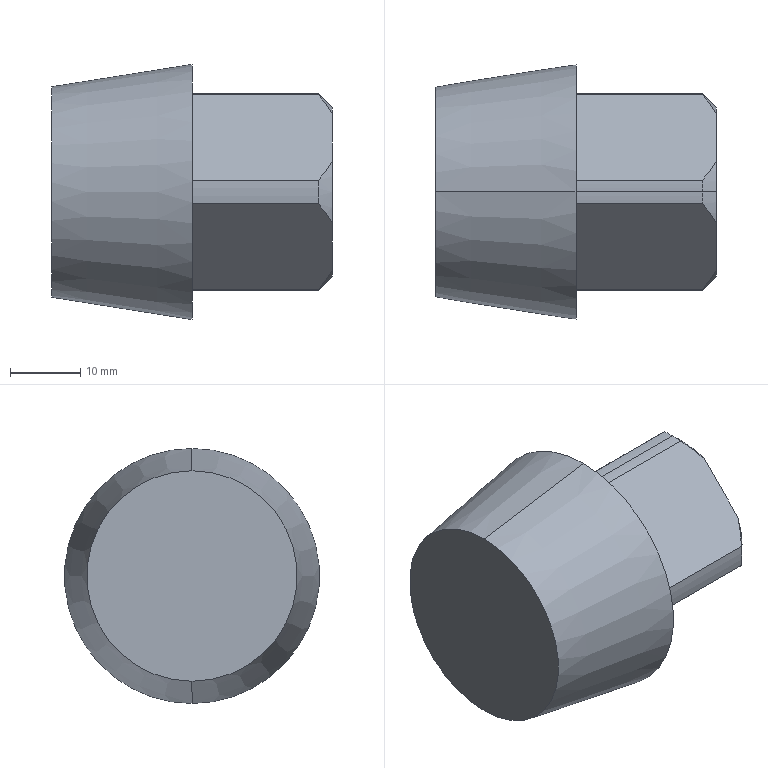Part | SolidWorks | features Chamfer 1, CirPattern 1, ICE 1, Revolution 1 | 1 solid | 19 faces | box 40 x 36.354 x 36.354 mm | volume 26781 mm3 | cone 7 | plane 7 | cylinder 5 | commonest cylinder face diameters 28 x5
STEP:
#1=CARTESIAN_POINT('',(0.,0.,15.));
#2=VERTEX_POINT('',#1);
#3=CARTESIAN_POINT('',(0.,0.,-15.));
#4=VERTEX_POINT('',#3);
#5=CARTESIAN_POINT('',(0.,0.,0.));
#6=DIRECTION('',(-1.,0.,0.));
#7=DIRECTION('',(0.,0.,1.));
#8=AXIS2_PLACEMENT_3D('',#5,#6,#7);
#9=CIRCLE('',#8,15.);
#10=EDGE_CURVE('',#2,#4,#9,.T.);
#11=ORIENTED_EDGE('',*,*,#10,.F.);
#12=CARTESIAN_POINT('',(20.,0.,18.177));
#13=VERTEX_POINT('',#12);
#14=CARTESIAN_POINT('',(20.,0.,18.177));
#15=DIRECTION('',(0.9876,0.,0.1569));
#16=VECTOR('',#15,1000.);
#17=LINE('',#14,#16);
#18=EDGE_CURVE('',#2,#13,#17,.T.);
#19=ORIENTED_EDGE('',*,*,#18,.T.);
#20=CARTESIAN_POINT('',(20.,0.,-18.177));
#21=VERTEX_POINT('',#20);
#22=CARTESIAN_POINT('',(20.,0.,0.));
#23=DIRECTION('',(-1.,0.,0.));
#24=DIRECTION('',(0.,0.,1.));
#25=AXIS2_PLACEMENT_3D('',#22,#23,#24);
#26=CIRCLE('',#25,18.177);
#27=EDGE_CURVE('',#13,#21,#26,.T.);
#28=ORIENTED_EDGE('',*,*,#27,.T.);
#29=CARTESIAN_POINT('',(20.,0.,-18.177));
#30=DIRECTION('',(0.9876,0.,-0.1569));
#31=VECTOR('',#30,1000.);
#32=LINE('',#29,#31);
#33=EDGE_CURVE('',#4,#21,#32,.T.);
#34=ORIENTED_EDGE('',*,*,#33,.F.);
#35=EDGE_LOOP('',(#11,#19,#28,#34));
#36=FACE_OUTER_BOUND('',#35,.T.);
#37=CARTESIAN_POINT('',(20.,0.,0.));
#38=DIRECTION('',(1.,0.,0.));
#39=DIRECTION('',(0.,0.,-1.));
#40=AXIS2_PLACEMENT_3D('',#37,#38,#39);
#41=CONICAL_SURFACE('',#40,18.177,0.1575);
#42=ADVANCED_FACE('',(#36),#41,.T.);
#43=CARTESIAN_POINT('',(40.,0.,12.));
#44=VERTEX_POINT('',#43);
#45=CARTESIAN_POINT('',(40.,-4.387,11.169));
#46=VERTEX_POINT('',#45);
#47=CARTESIAN_POINT('',(40.,0.,0.));
#48=DIRECTION('',(1.,0.,0.));
#49=DIRECTION('',(0.,0.,1.));
#50=AXIS2_PLACEMENT_3D('',#47,#48,#49);
#51=CIRCLE('',#50,12.);
#52=EDGE_CURVE('',#44,#46,#51,.T.);
#53=ORIENTED_EDGE('',*,*,#52,.F.);
#54=CARTESIAN_POINT('',(38.,0.,14.));
#55=VERTEX_POINT('',#54);
#56=CARTESIAN_POINT('',(38.,0.,14.));
#57=DIRECTION('',(-0.7071,0.,0.7071));
#58=VECTOR('',#57,1000.);
#59=LINE('',#56,#58);
#60=EDGE_CURVE('',#44,#55,#59,.T.);
#61=ORIENTED_EDGE('',*,*,#60,.T.);
#62=CARTESIAN_POINT('',(38.,-1.654,13.902));
#63=VERTEX_POINT('',#62);
#64=CARTESIAN_POINT('',(38.,0.,0.));
#65=DIRECTION('',(-1.,0.,0.));
#66=DIRECTION('',(0.,0.,1.));
#67=AXIS2_PLACEMENT_3D('',#64,#65,#66);
#68=CIRCLE('',#67,14.);
#69=EDGE_CURVE('',#63,#55,#68,.T.);
#70=ORIENTED_EDGE('',*,*,#69,.F.);
#71=CARTESIAN_POINT('',(38.,-1.654,13.902));
#72=CARTESIAN_POINT('',(38.384,-2.093,13.463));
#73=CARTESIAN_POINT('',(38.748,-2.538,13.018));
#74=CARTESIAN_POINT('',(39.421,-3.447,12.109));
#75=CARTESIAN_POINT('',(39.731,-3.91,11.646));
#76=CARTESIAN_POINT('',(40.,-4.387,11.169));
#77=B_SPLINE_CURVE_WITH_KNOTS('',3,(#71,#72,#73,#74,#75,#76),.UNSPECIFIED.,.F.,.F.,(4,2,4),(0.000001156,0.002175,0.004349),.UNSPECIFIED.);
#78=EDGE_CURVE('',#63,#46,#77,.T.);
#79=ORIENTED_EDGE('',*,*,#78,.T.);
#80=EDGE_LOOP('',(#53,#61,#70,#79));
#81=FACE_OUTER_BOUND('',#80,.T.);
#82=CARTESIAN_POINT('',(38.,0.,0.));
#83=DIRECTION('',(-1.,0.,0.));
#84=DIRECTION('',(0.,0.,1.));
#85=AXIS2_PLACEMENT_3D('',#82,#83,#84);
#86=CONICAL_SURFACE('',#85,14.,0.7854);
#87=ADVANCED_FACE('',(#81),#86,.T.);
#88=ORIENTED_EDGE('',*,*,#69,.T.);
#89=CARTESIAN_POINT('',(20.,0.,14.));
#90=VERTEX_POINT('',#89);
#91=CARTESIAN_POINT('',(20.,0.,14.));
#92=DIRECTION('',(-1.,0.,0.));
#93=VECTOR('',#92,1000.);
#94=LINE('',#91,#93);
#95=EDGE_CURVE('',#55,#90,#94,.T.);
#96=ORIENTED_EDGE('',*,*,#95,.T.);
#97=CARTESIAN_POINT('',(20.,-1.654,13.902));
#98=VERTEX_POINT('',#97);
#99=CARTESIAN_POINT('',(20.,0.,0.));
#100=DIRECTION('',(-1.,0.,0.));
#101=DIRECTION('',(0.,0.,1.));
#102=AXIS2_PLACEMENT_3D('',#99,#100,#101);
#103=CIRCLE('',#102,14.);
#104=EDGE_CURVE('',#98,#90,#103,.T.);
#105=ORIENTED_EDGE('',*,*,#104,.F.);
#106=CARTESIAN_POINT('',(20.,-1.654,13.902));
#107=DIRECTION('',(1.,0.,0.));
#108=VECTOR('',#107,1000.);
#109=LINE('',#106,#108);
#110=EDGE_CURVE('',#98,#63,#109,.T.);
#111=ORIENTED_EDGE('',*,*,#110,.T.);
#112=EDGE_LOOP('',(#88,#96,#105,#111));
#113=FACE_OUTER_BOUND('',#112,.T.);
#114=CARTESIAN_POINT('',(20.,0.,0.));
#115=DIRECTION('',(-1.,0.,0.));
#116=DIRECTION('',(0.,0.,1.));
#117=AXIS2_PLACEMENT_3D('',#114,#115,#116);
#118=CYLINDRICAL_SURFACE('',#117,14.);
#119=ADVANCED_FACE('',(#113),#118,.T.);
#120=CARTESIAN_POINT('',(20.,-13.902,-1.654));
#121=VERTEX_POINT('',#120);
#122=CARTESIAN_POINT('',(38.,-13.902,-1.654));
#123=VERTEX_POINT('',#122);
#124=CARTESIAN_POINT('',(20.,-13.902,-1.654));
#125=DIRECTION('',(1.,0.,0.));
#126=VECTOR('',#125,1000.);
#127=LINE('',#124,#126);
#128=EDGE_CURVE('',#121,#123,#127,.T.);
#129=ORIENTED_EDGE('',*,*,#128,.T.);
#130=CARTESIAN_POINT('',(38.,-13.902,1.654));
#131=VERTEX_POINT('',#130);
#132=CARTESIAN_POINT('',(38.,0.,0.));
#133=DIRECTION('',(-1.,0.,0.));
#134=DIRECTION('',(0.,0.,1.));
#135=AXIS2_PLACEMENT_3D('',#132,#133,#134);
#136=CIRCLE('',#135,14.);
#137=EDGE_CURVE('',#123,#131,#136,.T.);
#138=ORIENTED_EDGE('',*,*,#137,.T.);
#139=CARTESIAN_POINT('',(20.,-13.902,1.654));
#140=VERTEX_POINT('',#139);
#141=CARTESIAN_POINT('',(20.,-13.902,1.654));
#142=DIRECTION('',(1.,0.,0.));
#143=VECTOR('',#142,1000.);
#144=LINE('',#141,#143);
#145=EDGE_CURVE('',#140,#131,#144,.T.);
#146=ORIENTED_EDGE('',*,*,#145,.F.);
#147=CARTESIAN_POINT('',(20.,0.,0.));
#148=DIRECTION('',(-1.,0.,0.));
#149=DIRECTION('',(0.,0.,1.));
#150=AXIS2_PLACEMENT_3D('',#147,#148,#149);
#151=CIRCLE('',#150,14.);
#152=EDGE_CURVE('',#121,#140,#151,.T.);
#153=ORIENTED_EDGE('',*,*,#152,.F.);
#154=EDGE_LOOP('',(#129,#138,#146,#153));
#155=FACE_OUTER_BOUND('',#154,.T.);
#156=CARTESIAN_POINT('',(20.,0.,0.));
#157=DIRECTION('',(-1.,0.,0.));
#158=DIRECTION('',(0.,0.,1.));
#159=AXIS2_PLACEMENT_3D('',#156,#157,#158);
#160=CYLINDRICAL_SURFACE('',#159,14.);
#161=ADVANCED_FACE('',(#155),#160,.T.);
#162=CARTESIAN_POINT('',(20.,-1.654,-13.902));
#163=VERTEX_POINT('',#162);
#164=CARTESIAN_POINT('',(38.,-1.654,-13.902));
#165=VERTEX_POINT('',#164);
#166=CARTESIAN_POINT('',(20.,-1.654,-13.902));
#167=DIRECTION('',(1.,0.,0.));
#168=VECTOR('',#167,1000.);
#169=LINE('',#166,#168);
#170=EDGE_CURVE('',#163,#165,#169,.T.);
#171=ORIENTED_EDGE('',*,*,#170,.F.);
#172=CARTESIAN_POINT('',(20.,1.654,-13.902));
#173=VERTEX_POINT('',#172);
#174=CARTESIAN_POINT('',(20.,0.,0.));
#175=DIRECTION('',(-1.,0.,0.));
#176=DIRECTION('',(0.,0.,1.));
#177=AXIS2_PLACEMENT_3D('',#174,#175,#176);
#178=CIRCLE('',#177,14.);
#179=EDGE_CURVE('',#173,#163,#178,.T.);
#180=ORIENTED_EDGE('',*,*,#179,.F.);
#181=CARTESIAN_POINT('',(38.,1.654,-13.902));
#182=VERTEX_POINT('',#181);
#183=CARTESIAN_POINT('',(20.,1.654,-13.902));
#184=DIRECTION('',(1.,0.,0.));
#185=VECTOR('',#184,1000.);
#186=LINE('',#183,#185);
#187=EDGE_CURVE('',#173,#182,#186,.T.);
#188=ORIENTED_EDGE('',*,*,#187,.T.);
#189=CARTESIAN_POINT('',(38.,0.,0.));
#190=DIRECTION('',(-1.,0.,0.));
#191=DIRECTION('',(0.,0.,1.));
#192=AXIS2_PLACEMENT_3D('',#189,#190,#191);
#193=CIRCLE('',#192,14.);
#194=EDGE_CURVE('',#182,#165,#193,.T.);
#195=ORIENTED_EDGE('',*,*,#194,.T.);
#196=EDGE_LOOP('',(#171,#180,#188,#195));
#197=FACE_OUTER_BOUND('',#196,.T.);
#198=CARTESIAN_POINT('',(20.,0.,0.));
#199=DIRECTION('',(-1.,0.,0.));
#200=DIRECTION('',(0.,0.,1.));
#201=AXIS2_PLACEMENT_3D('',#198,#199,#200);
#202=CYLINDRICAL_SURFACE('',#201,14.);
#203=ADVANCED_FACE('',(#197),#202,.T.);
#204=ORIENTED_EDGE('',*,*,#95,.F.);
#205=CARTESIAN_POINT('',(38.,1.654,13.902));
#206=VERTEX_POINT('',#205);
#207=CARTESIAN_POINT('',(38.,0.,0.));
#208=DIRECTION('',(-1.,0.,0.));
#209=DIRECTION('',(0.,0.,1.));
#210=AXIS2_PLACEMENT_3D('',#207,#208,#209);
#211=CIRCLE('',#210,14.);
#212=EDGE_CURVE('',#55,#206,#211,.T.);
#213=ORIENTED_EDGE('',*,*,#212,.T.);
#214=CARTESIAN_POINT('',(20.,1.654,13.902));
#215=VERTEX_POINT('',#214);
#216=CARTESIAN_POINT('',(20.,1.654,13.902));
#217=DIRECTION('',(1.,0.,0.));
#218=VECTOR('',#217,1000.);
#219=LINE('',#216,#218);
#220=EDGE_CURVE('',#215,#206,#219,.T.);
#221=ORIENTED_EDGE('',*,*,#220,.F.);
#222=CARTESIAN_POINT('',(20.,0.,0.));
#223=DIRECTION('',(-1.,0.,0.));
#224=DIRECTION('',(0.,0.,1.));
#225=AXIS2_PLACEMENT_3D('',#222,#223,#224);
#226=CIRCLE('',#225,14.);
#227=EDGE_CURVE('',#90,#215,#226,.T.);
#228=ORIENTED_EDGE('',*,*,#227,.F.);
#229=EDGE_LOOP('',(#204,#213,#221,#228));
#230=FACE_OUTER_BOUND('',#229,.T.);
#231=CARTESIAN_POINT('',(20.,0.,0.));
#232=DIRECTION('',(-1.,0.,0.));
#233=DIRECTION('',(0.,0.,1.));
#234=AXIS2_PLACEMENT_3D('',#231,#232,#233);
#235=CYLINDRICAL_SURFACE('',#234,14.);
#236=ADVANCED_FACE('',(#230),#235,.T.);
#237=CARTESIAN_POINT('',(20.,13.902,1.654));
#238=VERTEX_POINT('',#237);
#239=CARTESIAN_POINT('',(38.,13.902,1.654));
#240=VERTEX_POINT('',#239);
#241=CARTESIAN_POINT('',(20.,13.902,1.654));
#242=DIRECTION('',(1.,0.,0.));
#243=VECTOR('',#242,1000.);
#244=LINE('',#241,#243);
#245=EDGE_CURVE('',#238,#240,#244,.T.);
#246=ORIENTED_EDGE('',*,*,#245,.T.);
#247=CARTESIAN_POINT('',(38.,13.902,-1.654));
#248=VERTEX_POINT('',#247);
#249=CARTESIAN_POINT('',(38.,0.,0.));
#250=DIRECTION('',(-1.,0.,0.));
#251=DIRECTION('',(0.,0.,1.));
#252=AXIS2_PLACEMENT_3D('',#249,#250,#251);
#253=CIRCLE('',#252,14.);
#254=EDGE_CURVE('',#240,#248,#253,.T.);
#255=ORIENTED_EDGE('',*,*,#254,.T.);
#256=CARTESIAN_POINT('',(20.,13.902,-1.654));
#257=VERTEX_POINT('',#256);
#258=CARTESIAN_POINT('',(20.,13.902,-1.654));
#259=DIRECTION('',(1.,0.,0.));
#260=VECTOR('',#259,1000.);
#261=LINE('',#258,#260);
#262=EDGE_CURVE('',#257,#248,#261,.T.);
#263=ORIENTED_EDGE('',*,*,#262,.F.);
#264=CARTESIAN_POINT('',(20.,0.,0.));
#265=DIRECTION('',(-1.,0.,0.));
#266=DIRECTION('',(0.,0.,1.));
#267=AXIS2_PLACEMENT_3D('',#264,#265,#266);
#268=CIRCLE('',#267,14.);
#269=EDGE_CURVE('',#238,#257,#268,.T.);
#270=ORIENTED_EDGE('',*,*,#269,.F.);
#271=EDGE_LOOP('',(#246,#255,#263,#270));
#272=FACE_OUTER_BOUND('',#271,.T.);
#273=CARTESIAN_POINT('',(20.,0.,0.));
#274=DIRECTION('',(-1.,0.,0.));
#275=DIRECTION('',(0.,0.,1.));
#276=AXIS2_PLACEMENT_3D('',#273,#274,#275);
#277=CYLINDRICAL_SURFACE('',#276,14.);
#278=ADVANCED_FACE('',(#272),#277,.T.);
#279=CARTESIAN_POINT('',(40.,-11.169,-4.387));
#280=VERTEX_POINT('',#279);
#281=CARTESIAN_POINT('',(40.,-4.387,-11.169));
#282=VERTEX_POINT('',#281);
#283=CARTESIAN_POINT('',(40.,-7.778,-7.778));
#284=DIRECTION('',(0.,0.7071,-0.7071));
#285=VECTOR('',#284,1000.);
#286=LINE('',#283,#285);
#287=EDGE_CURVE('',#280,#282,#286,.T.);
#288=ORIENTED_EDGE('',*,*,#287,.T.);
#289=CARTESIAN_POINT('',(40.,4.387,-11.169));
#290=VERTEX_POINT('',#289);
#291=CARTESIAN_POINT('',(40.,0.,0.));
#292=DIRECTION('',(1.,0.,0.));
#293=DIRECTION('',(0.,0.,1.));
#294=AXIS2_PLACEMENT_3D('',#291,#292,#293);
#295=CIRCLE('',#294,12.);
#296=EDGE_CURVE('',#282,#290,#295,.T.);
#297=ORIENTED_EDGE('',*,*,#296,.T.);
#298=CARTESIAN_POINT('',(40.,11.169,-4.387));
#299=VERTEX_POINT('',#298);
#300=CARTESIAN_POINT('',(40.,7.778,-7.778));
#301=DIRECTION('',(0.,0.7071,0.7071));
#302=VECTOR('',#301,1000.);
#303=LINE('',#300,#302);
#304=EDGE_CURVE('',#290,#299,#303,.T.);
#305=ORIENTED_EDGE('',*,*,#304,.T.);
#306=CARTESIAN_POINT('',(40.,11.169,4.387));
#307=VERTEX_POINT('',#306);
#308=CARTESIAN_POINT('',(40.,0.,0.));
#309=DIRECTION('',(1.,0.,0.));
#310=DIRECTION('',(0.,0.,1.));
#311=AXIS2_PLACEMENT_3D('',#308,#309,#310);
#312=CIRCLE('',#311,12.);
#313=EDGE_CURVE('',#299,#307,#312,.T.);
#314=ORIENTED_EDGE('',*,*,#313,.T.);
#315=CARTESIAN_POINT('',(40.,4.387,11.169));
#316=VERTEX_POINT('',#315);
#317=CARTESIAN_POINT('',(40.,7.778,7.778));
#318=DIRECTION('',(0.,-0.7071,0.7071));
#319=VECTOR('',#318,1000.);
#320=LINE('',#317,#319);
#321=EDGE_CURVE('',#307,#316,#320,.T.);
#322=ORIENTED_EDGE('',*,*,#321,.T.);
#323=CARTESIAN_POINT('',(40.,0.,0.));
#324=DIRECTION('',(1.,0.,0.));
#325=DIRECTION('',(0.,0.,1.));
#326=AXIS2_PLACEMENT_3D('',#323,#324,#325);
#327=CIRCLE('',#326,12.);
#328=EDGE_CURVE('',#316,#44,#327,.T.);
#329=ORIENTED_EDGE('',*,*,#328,.T.);
#330=ORIENTED_EDGE('',*,*,#52,.T.);
#331=CARTESIAN_POINT('',(40.,-11.169,4.387));
#332=VERTEX_POINT('',#331);
#333=CARTESIAN_POINT('',(40.,-7.778,7.778));
#334=DIRECTION('',(0.,-0.7071,-0.7071));
#335=VECTOR('',#334,1000.);
#336=LINE('',#333,#335);
#337=EDGE_CURVE('',#46,#332,#336,.T.);
#338=ORIENTED_EDGE('',*,*,#337,.T.);
#339=CARTESIAN_POINT('',(40.,0.,0.));
#340=DIRECTION('',(1.,0.,0.));
#341=DIRECTION('',(0.,0.,1.));
#342=AXIS2_PLACEMENT_3D('',#339,#340,#341);
#343=CIRCLE('',#342,12.);
#344=EDGE_CURVE('',#332,#280,#343,.T.);
#345=ORIENTED_EDGE('',*,*,#344,.T.);
#346=EDGE_LOOP('',(#288,#297,#305,#314,#322,#329,#330,#338,#345));
#347=FACE_OUTER_BOUND('',#346,.T.);
#348=CARTESIAN_POINT('',(40.,0.,0.));
#349=DIRECTION('',(-1.,0.,0.));
#350=DIRECTION('',(0.,0.,1.));
#351=AXIS2_PLACEMENT_3D('',#348,#349,#350);
#352=PLANE('',#351);
#353=ADVANCED_FACE('',(#347),#352,.F.);
#354=ORIENTED_EDGE('',*,*,#137,.F.);
#355=CARTESIAN_POINT('',(38.,-13.902,-1.654));
#356=CARTESIAN_POINT('',(38.384,-13.463,-2.093));
#357=CARTESIAN_POINT('',(38.748,-13.018,-2.538));
#358=CARTESIAN_POINT('',(39.421,-12.109,-3.447));
#359=CARTESIAN_POINT('',(39.731,-11.646,-3.91));
#360=CARTESIAN_POINT('',(40.,-11.169,-4.387));
#361=B_SPLINE_CURVE_WITH_KNOTS('',3,(#355,#356,#357,#358,#359,#360),.UNSPECIFIED.,.F.,.F.,(4,2,4),(0.000001156,0.002175,0.004349),.UNSPECIFIED.);
#362=EDGE_CURVE('',#123,#280,#361,.T.);
#363=ORIENTED_EDGE('',*,*,#362,.T.);
#364=ORIENTED_EDGE('',*,*,#344,.F.);
#365=CARTESIAN_POINT('',(40.,-11.169,4.387));
#366=CARTESIAN_POINT('',(39.73,-11.648,3.909));
#367=CARTESIAN_POINT('',(39.42,-12.111,3.445));
#368=CARTESIAN_POINT('',(38.747,-13.02,2.536));
#369=CARTESIAN_POINT('',(38.383,-13.464,2.092));
#370=CARTESIAN_POINT('',(38.,-13.902,1.654));
#371=B_SPLINE_CURVE_WITH_KNOTS('',3,(#365,#366,#367,#368,#369,#370),.UNSPECIFIED.,.F.,.F.,(4,2,4),(0.01415,0.01632,0.01848),.UNSPECIFIED.);
#372=EDGE_CURVE('',#332,#131,#371,.T.);
#373=ORIENTED_EDGE('',*,*,#372,.T.);
#374=EDGE_LOOP('',(#354,#363,#364,#373));
#375=FACE_OUTER_BOUND('',#374,.T.);
#376=CARTESIAN_POINT('',(38.,0.,0.));
#377=DIRECTION('',(-1.,0.,0.));
#378=DIRECTION('',(0.,0.,1.));
#379=AXIS2_PLACEMENT_3D('',#376,#377,#378);
#380=CONICAL_SURFACE('',#379,14.,0.7854);
#381=ADVANCED_FACE('',(#375),#380,.T.);
#382=ORIENTED_EDGE('',*,*,#296,.F.);
#383=CARTESIAN_POINT('',(40.,-4.387,-11.169));
#384=CARTESIAN_POINT('',(39.73,-3.909,-11.648));
#385=CARTESIAN_POINT('',(39.42,-3.445,-12.111));
#386=CARTESIAN_POINT('',(38.747,-2.536,-13.02));
#387=CARTESIAN_POINT('',(38.383,-2.092,-13.464));
#388=CARTESIAN_POINT('',(38.,-1.654,-13.902));
#389=B_SPLINE_CURVE_WITH_KNOTS('',3,(#383,#384,#385,#386,#387,#388),.UNSPECIFIED.,.F.,.F.,(4,2,4),(0.01415,0.01632,0.01848),.UNSPECIFIED.);
#390=EDGE_CURVE('',#282,#165,#389,.T.);
#391=ORIENTED_EDGE('',*,*,#390,.T.);
#392=ORIENTED_EDGE('',*,*,#194,.F.);
#393=CARTESIAN_POINT('',(38.,1.654,-13.902));
#394=CARTESIAN_POINT('',(38.384,2.093,-13.463));
#395=CARTESIAN_POINT('',(38.748,2.538,-13.018));
#396=CARTESIAN_POINT('',(39.421,3.447,-12.109));
#397=CARTESIAN_POINT('',(39.731,3.91,-11.646));
#398=CARTESIAN_POINT('',(40.,4.387,-11.169));
#399=B_SPLINE_CURVE_WITH_KNOTS('',3,(#393,#394,#395,#396,#397,#398),.UNSPECIFIED.,.F.,.F.,(4,2,4),(0.000001156,0.002175,0.004349),.UNSPECIFIED.);
#400=EDGE_CURVE('',#182,#290,#399,.T.);
#401=ORIENTED_EDGE('',*,*,#400,.T.);
#402=EDGE_LOOP('',(#382,#391,#392,#401));
#403=FACE_OUTER_BOUND('',#402,.T.);
#404=CARTESIAN_POINT('',(38.,0.,0.));
#405=DIRECTION('',(-1.,0.,0.));
#406=DIRECTION('',(0.,0.,1.));
#407=AXIS2_PLACEMENT_3D('',#404,#405,#406);
#408=CONICAL_SURFACE('',#407,14.,0.7854);
#409=ADVANCED_FACE('',(#403),#408,.T.);
#410=ORIENTED_EDGE('',*,*,#60,.F.);
#411=ORIENTED_EDGE('',*,*,#328,.F.);
#412=CARTESIAN_POINT('',(40.,4.387,11.169));
#413=CARTESIAN_POINT('',(39.73,3.909,11.648));
#414=CARTESIAN_POINT('',(39.42,3.445,12.111));
#415=CARTESIAN_POINT('',(38.747,2.536,13.02));
#416=CARTESIAN_POINT('',(38.383,2.092,13.464));
#417=CARTESIAN_POINT('',(38.,1.654,13.902));
#418=B_SPLINE_CURVE_WITH_KNOTS('',3,(#412,#413,#414,#415,#416,#417),.UNSPECIFIED.,.F.,.F.,(4,2,4),(0.01415,0.01632,0.01848),.UNSPECIFIED.);
#419=EDGE_CURVE('',#316,#206,#418,.T.);
#420=ORIENTED_EDGE('',*,*,#419,.T.);
#421=ORIENTED_EDGE('',*,*,#212,.F.);
#422=EDGE_LOOP('',(#410,#411,#420,#421));
#423=FACE_OUTER_BOUND('',#422,.T.);
#424=CARTESIAN_POINT('',(38.,0.,0.));
#425=DIRECTION('',(-1.,0.,0.));
#426=DIRECTION('',(0.,0.,1.));
#427=AXIS2_PLACEMENT_3D('',#424,#425,#426);
#428=CONICAL_SURFACE('',#427,14.,0.7854);
#429=ADVANCED_FACE('',(#423),#428,.T.);
#430=ORIENTED_EDGE('',*,*,#254,.F.);
#431=CARTESIAN_POINT('',(38.,13.902,1.654));
#432=CARTESIAN_POINT('',(38.384,13.463,2.093));
#433=CARTESIAN_POINT('',(38.748,13.018,2.538));
#434=CARTESIAN_POINT('',(39.421,12.109,3.447));
#435=CARTESIAN_POINT('',(39.731,11.646,3.91));
#436=CARTESIAN_POINT('',(40.,11.169,4.387));
#437=B_SPLINE_CURVE_WITH_KNOTS('',3,(#431,#432,#433,#434,#435,#436),.UNSPECIFIED.,.F.,.F.,(4,2,4),(0.000001156,0.002175,0.004349),.UNSPECIFIED.);
#438=EDGE_CURVE('',#240,#307,#437,.T.);
#439=ORIENTED_EDGE('',*,*,#438,.T.);
#440=ORIENTED_EDGE('',*,*,#313,.F.);
#441=CARTESIAN_POINT('',(40.,11.169,-4.387));
#442=CARTESIAN_POINT('',(39.73,11.648,-3.909));
#443=CARTESIAN_POINT('',(39.42,12.111,-3.445));
#444=CARTESIAN_POINT('',(38.747,13.02,-2.536));
#445=CARTESIAN_POINT('',(38.383,13.464,-2.092));
#446=CARTESIAN_POINT('',(38.,13.902,-1.654));
#447=B_SPLINE_CURVE_WITH_KNOTS('',3,(#441,#442,#443,#444,#445,#446),.UNSPECIFIED.,.F.,.F.,(4,2,4),(0.01415,0.01632,0.01848),.UNSPECIFIED.);
#448=EDGE_CURVE('',#299,#248,#447,.T.);
#449=ORIENTED_EDGE('',*,*,#448,.T.);
#450=EDGE_LOOP('',(#430,#439,#440,#449));
#451=FACE_OUTER_BOUND('',#450,.T.);
#452=CARTESIAN_POINT('',(38.,0.,0.));
#453=DIRECTION('',(-1.,0.,0.));
#454=DIRECTION('',(0.,0.,1.));
#455=AXIS2_PLACEMENT_3D('',#452,#453,#454);
#456=CONICAL_SURFACE('',#455,14.,0.7854);
#457=ADVANCED_FACE('',(#451),#456,.T.);
#458=CARTESIAN_POINT('',(0.,0.,0.));
#459=DIRECTION('',(-1.,0.,0.));
#460=DIRECTION('',(0.,0.,1.));
#461=AXIS2_PLACEMENT_3D('',#458,#459,#460);
#462=CIRCLE('',#461,15.);
#463=EDGE_CURVE('',#4,#2,#462,.T.);
#464=ORIENTED_EDGE('',*,*,#463,.T.);
#465=ORIENTED_EDGE('',*,*,#10,.T.);
#466=EDGE_LOOP('',(#464,#465));
#467=FACE_OUTER_BOUND('',#466,.T.);
#468=CARTESIAN_POINT('',(0.,0.,0.));
#469=DIRECTION('',(1.,0.,0.));
#470=DIRECTION('',(0.,0.,-1.));
#471=AXIS2_PLACEMENT_3D('',#468,#469,#470);
#472=PLANE('',#471);
#473=ADVANCED_FACE('',(#467),#472,.F.);
#474=ORIENTED_EDGE('',*,*,#18,.F.);
#475=ORIENTED_EDGE('',*,*,#463,.F.);
#476=ORIENTED_EDGE('',*,*,#33,.T.);
#477=CARTESIAN_POINT('',(20.,0.,0.));
#478=DIRECTION('',(-1.,0.,0.));
#479=DIRECTION('',(0.,0.,1.));
#480=AXIS2_PLACEMENT_3D('',#477,#478,#479);
#481=CIRCLE('',#480,18.177);
#482=EDGE_CURVE('',#21,#13,#481,.T.);
#483=ORIENTED_EDGE('',*,*,#482,.T.);
#484=EDGE_LOOP('',(#474,#475,#476,#483));
#485=FACE_OUTER_BOUND('',#484,.T.);
#486=CARTESIAN_POINT('',(20.,0.,0.));
#487=DIRECTION('',(1.,0.,0.));
#488=DIRECTION('',(0.,0.,-1.));
#489=AXIS2_PLACEMENT_3D('',#486,#487,#488);
#490=CONICAL_SURFACE('',#489,18.177,0.1575);
#491=ADVANCED_FACE('',(#485),#490,.T.);
#492=ORIENTED_EDGE('',*,*,#482,.F.);
#493=ORIENTED_EDGE('',*,*,#27,.F.);
#494=EDGE_LOOP('',(#492,#493));
#495=FACE_OUTER_BOUND('',#494,.T.);
#496=ORIENTED_EDGE('',*,*,#179,.T.);
#497=CARTESIAN_POINT('',(20.,-7.778,-7.778));
#498=DIRECTION('',(0.,0.7071,-0.7071));
#499=VECTOR('',#498,1000.);
#500=LINE('',#497,#499);
#501=EDGE_CURVE('',#121,#163,#500,.T.);
#502=ORIENTED_EDGE('',*,*,#501,.F.);
#503=ORIENTED_EDGE('',*,*,#152,.T.);
#504=CARTESIAN_POINT('',(20.,-7.778,7.778));
#505=DIRECTION('',(0.,-0.7071,-0.7071));
#506=VECTOR('',#505,1000.);
#507=LINE('',#504,#506);
#508=EDGE_CURVE('',#98,#140,#507,.T.);
#509=ORIENTED_EDGE('',*,*,#508,.F.);
#510=ORIENTED_EDGE('',*,*,#104,.T.);
#511=ORIENTED_EDGE('',*,*,#227,.T.);
#512=CARTESIAN_POINT('',(20.,7.778,7.778));
#513=DIRECTION('',(0.,-0.7071,0.7071));
#514=VECTOR('',#513,1000.);
#515=LINE('',#512,#514);
#516=EDGE_CURVE('',#238,#215,#515,.T.);
#517=ORIENTED_EDGE('',*,*,#516,.F.);
#518=ORIENTED_EDGE('',*,*,#269,.T.);
#519=CARTESIAN_POINT('',(20.,7.778,-7.778));
#520=DIRECTION('',(0.,0.7071,0.7071));
#521=VECTOR('',#520,1000.);
#522=LINE('',#519,#521);
#523=EDGE_CURVE('',#173,#257,#522,.T.);
#524=ORIENTED_EDGE('',*,*,#523,.F.);
#525=EDGE_LOOP('',(#496,#502,#503,#509,#510,#511,#517,#518,#524));
#526=FACE_BOUND('',#525,.T.);
#527=CARTESIAN_POINT('',(20.,14.,0.));
#528=DIRECTION('',(-1.,0.,0.));
#529=DIRECTION('',(0.,0.,1.));
#530=AXIS2_PLACEMENT_3D('',#527,#528,#529);
#531=PLANE('',#530);
#532=ADVANCED_FACE('',(#495,#526),#531,.F.);
#533=ORIENTED_EDGE('',*,*,#187,.F.);
#534=ORIENTED_EDGE('',*,*,#523,.T.);
#535=ORIENTED_EDGE('',*,*,#262,.T.);
#536=ORIENTED_EDGE('',*,*,#448,.F.);
#537=ORIENTED_EDGE('',*,*,#304,.F.);
#538=ORIENTED_EDGE('',*,*,#400,.F.);
#539=EDGE_LOOP('',(#533,#534,#535,#536,#537,#538));
#540=FACE_OUTER_BOUND('',#539,.T.);
#541=CARTESIAN_POINT('',(20.,7.778,-7.778));
#542=DIRECTION('',(0.,0.7071,-0.7071));
#543=DIRECTION('',(0.,0.7071,0.7071));
#544=AXIS2_PLACEMENT_3D('',#541,#542,#543);
#545=PLANE('',#544);
#546=ADVANCED_FACE('',(#540),#545,.T.);
#547=ORIENTED_EDGE('',*,*,#245,.F.);
#548=ORIENTED_EDGE('',*,*,#516,.T.);
#549=ORIENTED_EDGE('',*,*,#220,.T.);
#550=ORIENTED_EDGE('',*,*,#419,.F.);
#551=ORIENTED_EDGE('',*,*,#321,.F.);
#552=ORIENTED_EDGE('',*,*,#438,.F.);
#553=EDGE_LOOP('',(#547,#548,#549,#550,#551,#552));
#554=FACE_OUTER_BOUND('',#553,.T.);
#555=CARTESIAN_POINT('',(20.,7.778,7.778));
#556=DIRECTION('',(0.,0.7071,0.7071));
#557=DIRECTION('',(0.,-0.7071,0.7071));
#558=AXIS2_PLACEMENT_3D('',#555,#556,#557);
#559=PLANE('',#558);
#560=ADVANCED_FACE('',(#554),#559,.T.);
#561=ORIENTED_EDGE('',*,*,#110,.F.);
#562=ORIENTED_EDGE('',*,*,#508,.T.);
#563=ORIENTED_EDGE('',*,*,#145,.T.);
#564=ORIENTED_EDGE('',*,*,#372,.F.);
#565=ORIENTED_EDGE('',*,*,#337,.F.);
#566=ORIENTED_EDGE('',*,*,#78,.F.);
#567=EDGE_LOOP('',(#561,#562,#563,#564,#565,#566));
#568=FACE_OUTER_BOUND('',#567,.T.);
#569=CARTESIAN_POINT('',(20.,-7.778,7.778));
#570=DIRECTION('',(0.,-0.7071,0.7071));
#571=DIRECTION('',(0.,-0.7071,-0.7071));
#572=AXIS2_PLACEMENT_3D('',#569,#570,#571);
#573=PLANE('',#572);
#574=ADVANCED_FACE('',(#568),#573,.T.);
#575=ORIENTED_EDGE('',*,*,#128,.F.);
#576=ORIENTED_EDGE('',*,*,#501,.T.);
#577=ORIENTED_EDGE('',*,*,#170,.T.);
#578=ORIENTED_EDGE('',*,*,#390,.F.);
#579=ORIENTED_EDGE('',*,*,#287,.F.);
#580=ORIENTED_EDGE('',*,*,#362,.F.);
#581=EDGE_LOOP('',(#575,#576,#577,#578,#579,#580));
#582=FACE_OUTER_BOUND('',#581,.T.);
#583=CARTESIAN_POINT('',(20.,-7.778,-7.778));
#584=DIRECTION('',(0.,-0.7071,-0.7071));
#585=DIRECTION('',(0.,0.7071,-0.7071));
#586=AXIS2_PLACEMENT_3D('',#583,#584,#585);
#587=PLANE('',#586);
#588=ADVANCED_FACE('',(#582),#587,.T.);
#589=CLOSED_SHELL('',(#42,#87,#119,#161,#203,#236,#278,#353,#381,#409,#429,#457,#473,#491,#532,#546,#560,#574,#588));
#590=MANIFOLD_SOLID_BREP('',#589);
#591=CARTESIAN_POINT('',(0.,0.,0.));
#592=DIRECTION('',(0.,0.,1.));
#593=DIRECTION('',(1.,0.,0.));
#594=AXIS2_PLACEMENT_3D('',#591,#592,#593);
#595=(LENGTH_UNIT()NAMED_UNIT(*)SI_UNIT(.MILLI.,.METRE.));
#596=UNCERTAINTY_MEASURE_WITH_UNIT(LENGTH_MEASURE(0.00001),#595,'','');
#597=(NAMED_UNIT(*)PLANE_ANGLE_UNIT()SI_UNIT($,.RADIAN.));
#598=(NAMED_UNIT(*)SI_UNIT($,.STERADIAN.)SOLID_ANGLE_UNIT());
#599=(GEOMETRIC_REPRESENTATION_CONTEXT(3)GLOBAL_UNCERTAINTY_ASSIGNED_CONTEXT((#596))GLOBAL_UNIT_ASSIGNED_CONTEXT((#595,#597,#598))REPRESENTATION_CONTEXT('',''));
#600=ADVANCED_BREP_SHAPE_REPRESENTATION('',(#590,#594),#599);